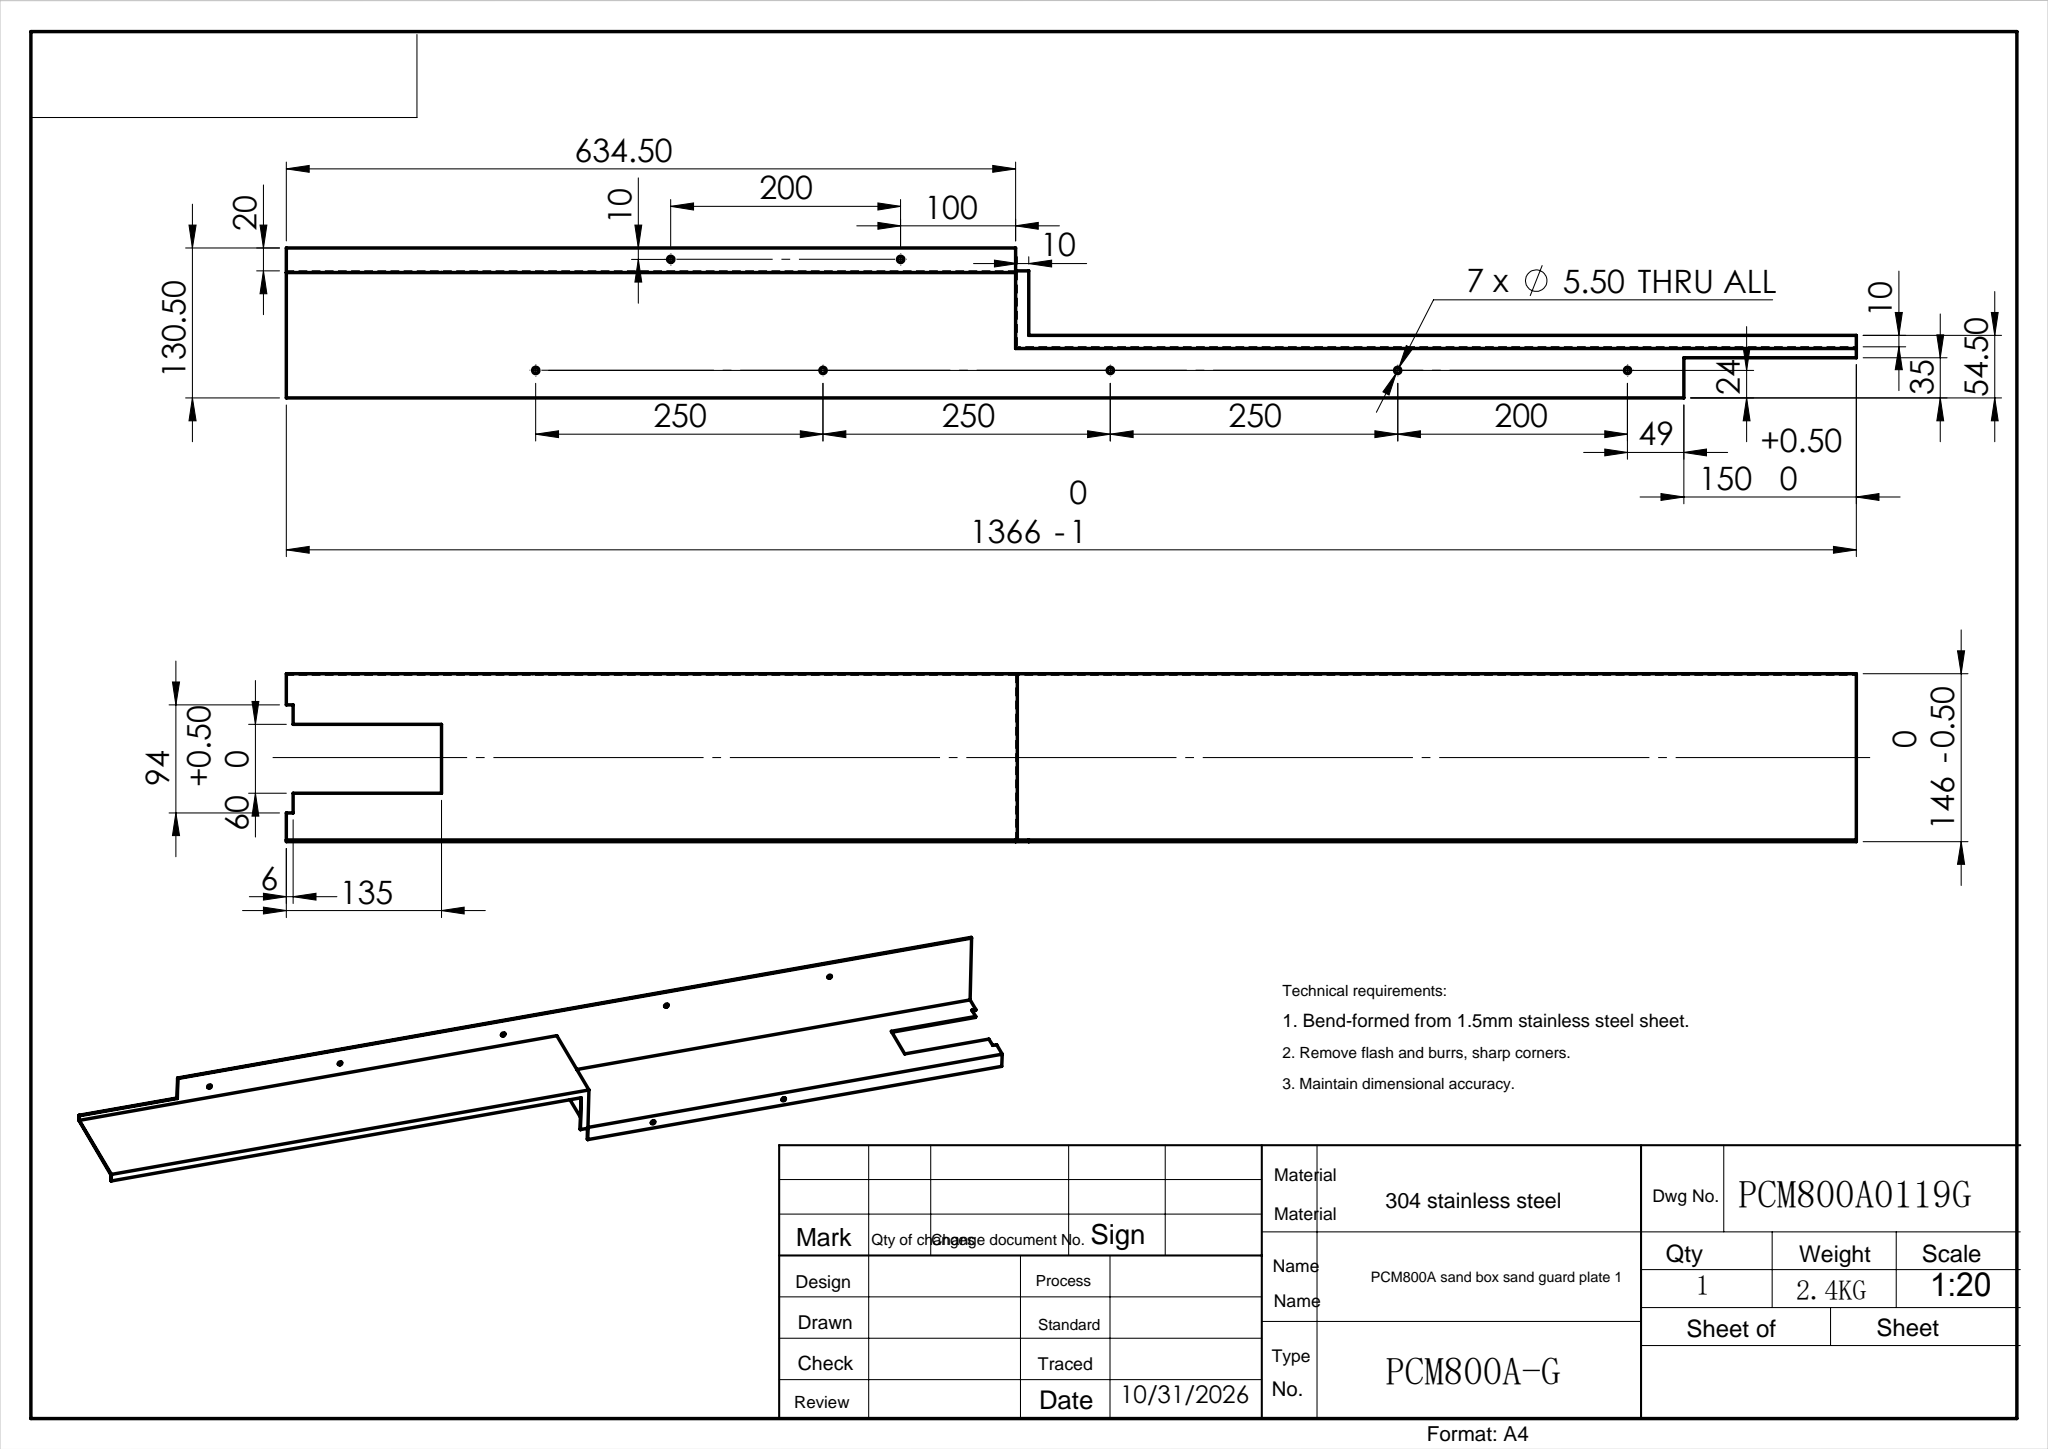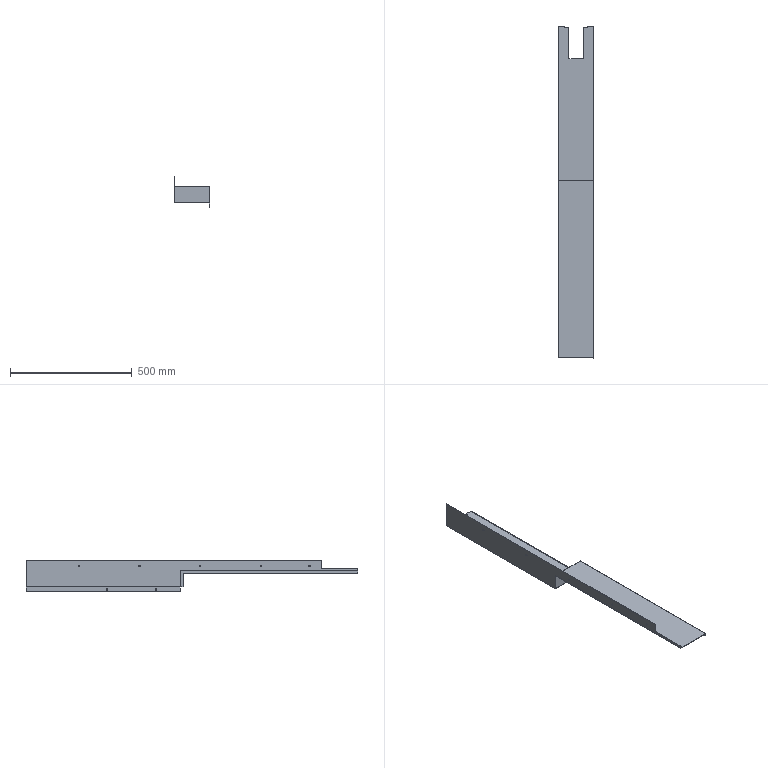Part | SolidWorks | features ICE 8, HoleWzd 2, Extrusion 1 | 1 solid | 42 faces | box 146 x 1366 x 130.5 mm | volume 474775 mm3 | plane 28 | cylinder 14 | commonest cylinder face diameters 5.5 x14